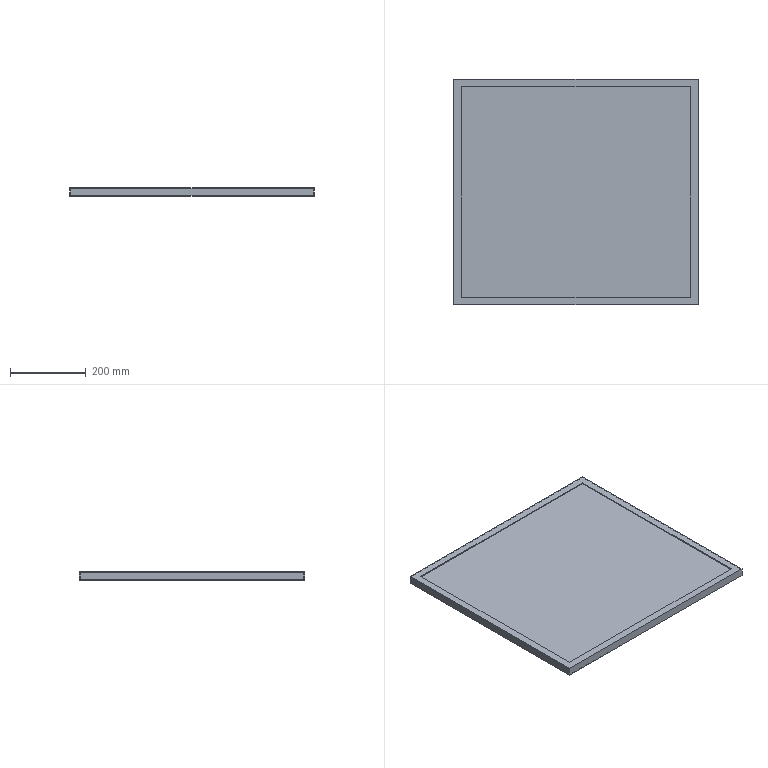Part | SolidWorks | features Extrusion 1, ICE 1, Shell 1 | 1 solid | 16 faces | box 645 x 596 x 22 mm | volume 953984 mm3 | plane 16
STEP:
#1=CARTESIAN_POINT('',(0.,596.,22.));
#2=VERTEX_POINT('',#1);
#3=CARTESIAN_POINT('',(0.,0.,22.));
#4=VERTEX_POINT('',#3);
#5=CARTESIAN_POINT('',(0.,0.,22.));
#6=DIRECTION('',(0.,-1.,0.));
#7=VECTOR('',#6,1000.);
#8=LINE('',#5,#7);
#9=EDGE_CURVE('',#2,#4,#8,.T.);
#10=ORIENTED_EDGE('',*,*,#9,.T.);
#11=CARTESIAN_POINT('',(645.,0.,22.));
#12=VERTEX_POINT('',#11);
#13=CARTESIAN_POINT('',(0.,0.,22.));
#14=DIRECTION('',(1.,0.,0.));
#15=VECTOR('',#14,1000.);
#16=LINE('',#13,#15);
#17=EDGE_CURVE('',#4,#12,#16,.T.);
#18=ORIENTED_EDGE('',*,*,#17,.T.);
#19=CARTESIAN_POINT('',(645.,596.,22.));
#20=VERTEX_POINT('',#19);
#21=CARTESIAN_POINT('',(645.,0.,22.));
#22=DIRECTION('',(0.,1.,0.));
#23=VECTOR('',#22,1000.);
#24=LINE('',#21,#23);
#25=EDGE_CURVE('',#12,#20,#24,.T.);
#26=ORIENTED_EDGE('',*,*,#25,.T.);
#27=CARTESIAN_POINT('',(0.,596.,22.));
#28=DIRECTION('',(-1.,0.,0.));
#29=VECTOR('',#28,1000.);
#30=LINE('',#27,#29);
#31=EDGE_CURVE('',#20,#2,#30,.T.);
#32=ORIENTED_EDGE('',*,*,#31,.T.);
#33=EDGE_LOOP('',(#10,#18,#26,#32));
#34=FACE_OUTER_BOUND('',#33,.T.);
#35=CARTESIAN_POINT('',(625.,576.,22.));
#36=VERTEX_POINT('',#35);
#37=CARTESIAN_POINT('',(20.,576.,22.));
#38=VERTEX_POINT('',#37);
#39=CARTESIAN_POINT('',(625.,576.,22.));
#40=DIRECTION('',(-1.,0.,0.));
#41=VECTOR('',#40,1000.);
#42=LINE('',#39,#41);
#43=EDGE_CURVE('',#36,#38,#42,.T.);
#44=ORIENTED_EDGE('',*,*,#43,.F.);
#45=CARTESIAN_POINT('',(625.,20.,22.));
#46=VERTEX_POINT('',#45);
#47=CARTESIAN_POINT('',(625.,20.,22.));
#48=DIRECTION('',(0.,1.,0.));
#49=VECTOR('',#48,1000.);
#50=LINE('',#47,#49);
#51=EDGE_CURVE('',#46,#36,#50,.T.);
#52=ORIENTED_EDGE('',*,*,#51,.F.);
#53=CARTESIAN_POINT('',(20.,20.,22.));
#54=VERTEX_POINT('',#53);
#55=CARTESIAN_POINT('',(20.,20.,22.));
#56=DIRECTION('',(1.,0.,0.));
#57=VECTOR('',#56,1000.);
#58=LINE('',#55,#57);
#59=EDGE_CURVE('',#54,#46,#58,.T.);
#60=ORIENTED_EDGE('',*,*,#59,.F.);
#61=CARTESIAN_POINT('',(20.,576.,22.));
#62=DIRECTION('',(0.,-1.,0.));
#63=VECTOR('',#62,1000.);
#64=LINE('',#61,#63);
#65=EDGE_CURVE('',#38,#54,#64,.T.);
#66=ORIENTED_EDGE('',*,*,#65,.F.);
#67=EDGE_LOOP('',(#44,#52,#60,#66));
#68=FACE_BOUND('',#67,.T.);
#69=CARTESIAN_POINT('',(0.,596.,22.));
#70=DIRECTION('',(0.,0.,-1.));
#71=DIRECTION('',(-1.,0.,0.));
#72=AXIS2_PLACEMENT_3D('',#69,#70,#71);
#73=PLANE('',#72);
#74=ADVANCED_FACE('',(#34,#68),#73,.F.);
#75=CARTESIAN_POINT('',(0.,596.,0.));
#76=VERTEX_POINT('',#75);
#77=CARTESIAN_POINT('',(0.,596.,22.));
#78=DIRECTION('',(0.,0.,-1.));
#79=VECTOR('',#78,1000.);
#80=LINE('',#77,#79);
#81=EDGE_CURVE('',#2,#76,#80,.T.);
#82=ORIENTED_EDGE('',*,*,#81,.T.);
#83=CARTESIAN_POINT('',(0.,0.,0.));
#84=VERTEX_POINT('',#83);
#85=CARTESIAN_POINT('',(0.,0.,0.));
#86=DIRECTION('',(0.,-1.,0.));
#87=VECTOR('',#86,1000.);
#88=LINE('',#85,#87);
#89=EDGE_CURVE('',#76,#84,#88,.T.);
#90=ORIENTED_EDGE('',*,*,#89,.T.);
#91=CARTESIAN_POINT('',(0.,0.,22.));
#92=DIRECTION('',(0.,0.,-1.));
#93=VECTOR('',#92,1000.);
#94=LINE('',#91,#93);
#95=EDGE_CURVE('',#4,#84,#94,.T.);
#96=ORIENTED_EDGE('',*,*,#95,.F.);
#97=ORIENTED_EDGE('',*,*,#9,.F.);
#98=EDGE_LOOP('',(#82,#90,#96,#97));
#99=FACE_OUTER_BOUND('',#98,.T.);
#100=CARTESIAN_POINT('',(0.,0.,22.));
#101=DIRECTION('',(1.,0.,0.));
#102=DIRECTION('',(0.,0.,-1.));
#103=AXIS2_PLACEMENT_3D('',#100,#101,#102);
#104=PLANE('',#103);
#105=ADVANCED_FACE('',(#99),#104,.F.);
#106=ORIENTED_EDGE('',*,*,#95,.T.);
#107=CARTESIAN_POINT('',(645.,0.,0.));
#108=VERTEX_POINT('',#107);
#109=CARTESIAN_POINT('',(0.,0.,0.));
#110=DIRECTION('',(1.,0.,0.));
#111=VECTOR('',#110,1000.);
#112=LINE('',#109,#111);
#113=EDGE_CURVE('',#84,#108,#112,.T.);
#114=ORIENTED_EDGE('',*,*,#113,.T.);
#115=CARTESIAN_POINT('',(645.,0.,22.));
#116=DIRECTION('',(0.,0.,-1.));
#117=VECTOR('',#116,1000.);
#118=LINE('',#115,#117);
#119=EDGE_CURVE('',#12,#108,#118,.T.);
#120=ORIENTED_EDGE('',*,*,#119,.F.);
#121=ORIENTED_EDGE('',*,*,#17,.F.);
#122=EDGE_LOOP('',(#106,#114,#120,#121));
#123=FACE_OUTER_BOUND('',#122,.T.);
#124=CARTESIAN_POINT('',(0.,0.,22.));
#125=DIRECTION('',(0.,1.,0.));
#126=DIRECTION('',(0.,0.,1.));
#127=AXIS2_PLACEMENT_3D('',#124,#125,#126);
#128=PLANE('',#127);
#129=ADVANCED_FACE('',(#123),#128,.F.);
#130=ORIENTED_EDGE('',*,*,#119,.T.);
#131=CARTESIAN_POINT('',(645.,596.,0.));
#132=VERTEX_POINT('',#131);
#133=CARTESIAN_POINT('',(645.,0.,0.));
#134=DIRECTION('',(0.,1.,0.));
#135=VECTOR('',#134,1000.);
#136=LINE('',#133,#135);
#137=EDGE_CURVE('',#108,#132,#136,.T.);
#138=ORIENTED_EDGE('',*,*,#137,.T.);
#139=CARTESIAN_POINT('',(645.,596.,22.));
#140=DIRECTION('',(0.,0.,-1.));
#141=VECTOR('',#140,1000.);
#142=LINE('',#139,#141);
#143=EDGE_CURVE('',#20,#132,#142,.T.);
#144=ORIENTED_EDGE('',*,*,#143,.F.);
#145=ORIENTED_EDGE('',*,*,#25,.F.);
#146=EDGE_LOOP('',(#130,#138,#144,#145));
#147=FACE_OUTER_BOUND('',#146,.T.);
#148=CARTESIAN_POINT('',(645.,0.,22.));
#149=DIRECTION('',(-1.,0.,0.));
#150=DIRECTION('',(0.,0.,1.));
#151=AXIS2_PLACEMENT_3D('',#148,#149,#150);
#152=PLANE('',#151);
#153=ADVANCED_FACE('',(#147),#152,.F.);
#154=ORIENTED_EDGE('',*,*,#143,.T.);
#155=CARTESIAN_POINT('',(0.,596.,0.));
#156=DIRECTION('',(-1.,0.,0.));
#157=VECTOR('',#156,1000.);
#158=LINE('',#155,#157);
#159=EDGE_CURVE('',#132,#76,#158,.T.);
#160=ORIENTED_EDGE('',*,*,#159,.T.);
#161=ORIENTED_EDGE('',*,*,#81,.F.);
#162=ORIENTED_EDGE('',*,*,#31,.F.);
#163=EDGE_LOOP('',(#154,#160,#161,#162));
#164=FACE_OUTER_BOUND('',#163,.T.);
#165=CARTESIAN_POINT('',(0.,596.,22.));
#166=DIRECTION('',(0.,-1.,0.));
#167=DIRECTION('',(0.,0.,-1.));
#168=AXIS2_PLACEMENT_3D('',#165,#166,#167);
#169=PLANE('',#168);
#170=ADVANCED_FACE('',(#164),#169,.F.);
#171=ORIENTED_EDGE('',*,*,#89,.F.);
#172=ORIENTED_EDGE('',*,*,#159,.F.);
#173=ORIENTED_EDGE('',*,*,#137,.F.);
#174=ORIENTED_EDGE('',*,*,#113,.F.);
#175=EDGE_LOOP('',(#171,#172,#173,#174));
#176=FACE_OUTER_BOUND('',#175,.T.);
#177=CARTESIAN_POINT('',(0.,596.,0.));
#178=DIRECTION('',(0.,0.,-1.));
#179=DIRECTION('',(-1.,0.,0.));
#180=AXIS2_PLACEMENT_3D('',#177,#178,#179);
#181=PLANE('',#180);
#182=ADVANCED_FACE('',(#176),#181,.T.);
#183=CARTESIAN_POINT('',(2.,594.,20.));
#184=VERTEX_POINT('',#183);
#185=CARTESIAN_POINT('',(2.,2.,20.));
#186=VERTEX_POINT('',#185);
#187=CARTESIAN_POINT('',(2.,0.,20.));
#188=DIRECTION('',(0.,-1.,0.));
#189=VECTOR('',#188,1000.);
#190=LINE('',#187,#189);
#191=EDGE_CURVE('',#184,#186,#190,.T.);
#192=ORIENTED_EDGE('',*,*,#191,.F.);
#193=CARTESIAN_POINT('',(643.,594.,20.));
#194=VERTEX_POINT('',#193);
#195=CARTESIAN_POINT('',(0.,594.,20.));
#196=DIRECTION('',(-1.,0.,0.));
#197=VECTOR('',#196,1000.);
#198=LINE('',#195,#197);
#199=EDGE_CURVE('',#194,#184,#198,.T.);
#200=ORIENTED_EDGE('',*,*,#199,.F.);
#201=CARTESIAN_POINT('',(643.,2.,20.));
#202=VERTEX_POINT('',#201);
#203=CARTESIAN_POINT('',(643.,0.,20.));
#204=DIRECTION('',(0.,1.,0.));
#205=VECTOR('',#204,1000.);
#206=LINE('',#203,#205);
#207=EDGE_CURVE('',#202,#194,#206,.T.);
#208=ORIENTED_EDGE('',*,*,#207,.F.);
#209=CARTESIAN_POINT('',(0.,2.,20.));
#210=DIRECTION('',(1.,0.,0.));
#211=VECTOR('',#210,1000.);
#212=LINE('',#209,#211);
#213=EDGE_CURVE('',#186,#202,#212,.T.);
#214=ORIENTED_EDGE('',*,*,#213,.F.);
#215=EDGE_LOOP('',(#192,#200,#208,#214));
#216=FACE_OUTER_BOUND('',#215,.T.);
#217=CARTESIAN_POINT('',(625.,20.,20.));
#218=VERTEX_POINT('',#217);
#219=CARTESIAN_POINT('',(625.,576.,20.));
#220=VERTEX_POINT('',#219);
#221=CARTESIAN_POINT('',(625.,20.,20.));
#222=DIRECTION('',(0.,1.,0.));
#223=VECTOR('',#222,1000.);
#224=LINE('',#221,#223);
#225=EDGE_CURVE('',#218,#220,#224,.T.);
#226=ORIENTED_EDGE('',*,*,#225,.T.);
#227=CARTESIAN_POINT('',(20.,576.,20.));
#228=VERTEX_POINT('',#227);
#229=CARTESIAN_POINT('',(625.,576.,20.));
#230=DIRECTION('',(-1.,0.,0.));
#231=VECTOR('',#230,1000.);
#232=LINE('',#229,#231);
#233=EDGE_CURVE('',#220,#228,#232,.T.);
#234=ORIENTED_EDGE('',*,*,#233,.T.);
#235=CARTESIAN_POINT('',(20.,20.,20.));
#236=VERTEX_POINT('',#235);
#237=CARTESIAN_POINT('',(20.,576.,20.));
#238=DIRECTION('',(0.,-1.,0.));
#239=VECTOR('',#238,1000.);
#240=LINE('',#237,#239);
#241=EDGE_CURVE('',#228,#236,#240,.T.);
#242=ORIENTED_EDGE('',*,*,#241,.T.);
#243=CARTESIAN_POINT('',(20.,20.,20.));
#244=DIRECTION('',(1.,0.,0.));
#245=VECTOR('',#244,1000.);
#246=LINE('',#243,#245);
#247=EDGE_CURVE('',#236,#218,#246,.T.);
#248=ORIENTED_EDGE('',*,*,#247,.T.);
#249=EDGE_LOOP('',(#226,#234,#242,#248));
#250=FACE_BOUND('',#249,.T.);
#251=CARTESIAN_POINT('',(0.,596.,20.));
#252=DIRECTION('',(0.,0.,1.));
#253=DIRECTION('',(1.,0.,0.));
#254=AXIS2_PLACEMENT_3D('',#251,#252,#253);
#255=PLANE('',#254);
#256=ADVANCED_FACE('',(#216,#250),#255,.F.);
#257=ORIENTED_EDGE('',*,*,#43,.T.);
#258=CARTESIAN_POINT('',(20.,576.,20.));
#259=DIRECTION('',(0.,0.,1.));
#260=VECTOR('',#259,1000.);
#261=LINE('',#258,#260);
#262=EDGE_CURVE('',#228,#38,#261,.T.);
#263=ORIENTED_EDGE('',*,*,#262,.F.);
#264=ORIENTED_EDGE('',*,*,#233,.F.);
#265=CARTESIAN_POINT('',(625.,576.,20.));
#266=DIRECTION('',(0.,0.,1.));
#267=VECTOR('',#266,1000.);
#268=LINE('',#265,#267);
#269=EDGE_CURVE('',#220,#36,#268,.T.);
#270=ORIENTED_EDGE('',*,*,#269,.T.);
#271=EDGE_LOOP('',(#257,#263,#264,#270));
#272=FACE_OUTER_BOUND('',#271,.T.);
#273=CARTESIAN_POINT('',(625.,576.,20.));
#274=DIRECTION('',(0.,1.,0.));
#275=DIRECTION('',(0.,0.,1.));
#276=AXIS2_PLACEMENT_3D('',#273,#274,#275);
#277=PLANE('',#276);
#278=ADVANCED_FACE('',(#272),#277,.F.);
#279=ORIENTED_EDGE('',*,*,#51,.T.);
#280=ORIENTED_EDGE('',*,*,#269,.F.);
#281=ORIENTED_EDGE('',*,*,#225,.F.);
#282=CARTESIAN_POINT('',(625.,20.,20.));
#283=DIRECTION('',(0.,0.,1.));
#284=VECTOR('',#283,1000.);
#285=LINE('',#282,#284);
#286=EDGE_CURVE('',#218,#46,#285,.T.);
#287=ORIENTED_EDGE('',*,*,#286,.T.);
#288=EDGE_LOOP('',(#279,#280,#281,#287));
#289=FACE_OUTER_BOUND('',#288,.T.);
#290=CARTESIAN_POINT('',(625.,20.,20.));
#291=DIRECTION('',(1.,0.,0.));
#292=DIRECTION('',(0.,0.,-1.));
#293=AXIS2_PLACEMENT_3D('',#290,#291,#292);
#294=PLANE('',#293);
#295=ADVANCED_FACE('',(#289),#294,.F.);
#296=ORIENTED_EDGE('',*,*,#59,.T.);
#297=ORIENTED_EDGE('',*,*,#286,.F.);
#298=ORIENTED_EDGE('',*,*,#247,.F.);
#299=CARTESIAN_POINT('',(20.,20.,20.));
#300=DIRECTION('',(0.,0.,1.));
#301=VECTOR('',#300,1000.);
#302=LINE('',#299,#301);
#303=EDGE_CURVE('',#236,#54,#302,.T.);
#304=ORIENTED_EDGE('',*,*,#303,.T.);
#305=EDGE_LOOP('',(#296,#297,#298,#304));
#306=FACE_OUTER_BOUND('',#305,.T.);
#307=CARTESIAN_POINT('',(20.,20.,20.));
#308=DIRECTION('',(0.,-1.,0.));
#309=DIRECTION('',(0.,0.,-1.));
#310=AXIS2_PLACEMENT_3D('',#307,#308,#309);
#311=PLANE('',#310);
#312=ADVANCED_FACE('',(#306),#311,.F.);
#313=ORIENTED_EDGE('',*,*,#65,.T.);
#314=ORIENTED_EDGE('',*,*,#303,.F.);
#315=ORIENTED_EDGE('',*,*,#241,.F.);
#316=ORIENTED_EDGE('',*,*,#262,.T.);
#317=EDGE_LOOP('',(#313,#314,#315,#316));
#318=FACE_OUTER_BOUND('',#317,.T.);
#319=CARTESIAN_POINT('',(20.,576.,20.));
#320=DIRECTION('',(-1.,0.,0.));
#321=DIRECTION('',(0.,0.,1.));
#322=AXIS2_PLACEMENT_3D('',#319,#320,#321);
#323=PLANE('',#322);
#324=ADVANCED_FACE('',(#318),#323,.F.);
#325=CARTESIAN_POINT('',(2.,594.,2.));
#326=VERTEX_POINT('',#325);
#327=CARTESIAN_POINT('',(2.,2.,2.));
#328=VERTEX_POINT('',#327);
#329=CARTESIAN_POINT('',(2.,596.,2.));
#330=DIRECTION('',(0.,-1.,0.));
#331=VECTOR('',#330,1000.);
#332=LINE('',#329,#331);
#333=EDGE_CURVE('',#326,#328,#332,.T.);
#334=ORIENTED_EDGE('',*,*,#333,.T.);
#335=CARTESIAN_POINT('',(643.,2.,2.));
#336=VERTEX_POINT('',#335);
#337=CARTESIAN_POINT('',(0.,2.,2.));
#338=DIRECTION('',(1.,0.,0.));
#339=VECTOR('',#338,1000.);
#340=LINE('',#337,#339);
#341=EDGE_CURVE('',#328,#336,#340,.T.);
#342=ORIENTED_EDGE('',*,*,#341,.T.);
#343=CARTESIAN_POINT('',(643.,594.,2.));
#344=VERTEX_POINT('',#343);
#345=CARTESIAN_POINT('',(643.,596.,2.));
#346=DIRECTION('',(0.,1.,0.));
#347=VECTOR('',#346,1000.);
#348=LINE('',#345,#347);
#349=EDGE_CURVE('',#336,#344,#348,.T.);
#350=ORIENTED_EDGE('',*,*,#349,.T.);
#351=CARTESIAN_POINT('',(0.,594.,2.));
#352=DIRECTION('',(-1.,0.,0.));
#353=VECTOR('',#352,1000.);
#354=LINE('',#351,#353);
#355=EDGE_CURVE('',#344,#326,#354,.T.);
#356=ORIENTED_EDGE('',*,*,#355,.T.);
#357=EDGE_LOOP('',(#334,#342,#350,#356));
#358=FACE_OUTER_BOUND('',#357,.T.);
#359=CARTESIAN_POINT('',(0.,596.,2.));
#360=DIRECTION('',(0.,0.,-1.));
#361=DIRECTION('',(-1.,0.,0.));
#362=AXIS2_PLACEMENT_3D('',#359,#360,#361);
#363=PLANE('',#362);
#364=ADVANCED_FACE('',(#358),#363,.F.);
#365=CARTESIAN_POINT('',(643.,594.,22.));
#366=DIRECTION('',(0.,0.,-1.));
#367=VECTOR('',#366,1000.);
#368=LINE('',#365,#367);
#369=EDGE_CURVE('',#194,#344,#368,.T.);
#370=ORIENTED_EDGE('',*,*,#369,.F.);
#371=ORIENTED_EDGE('',*,*,#199,.T.);
#372=CARTESIAN_POINT('',(2.,594.,22.));
#373=DIRECTION('',(0.,0.,-1.));
#374=VECTOR('',#373,1000.);
#375=LINE('',#372,#374);
#376=EDGE_CURVE('',#184,#326,#375,.T.);
#377=ORIENTED_EDGE('',*,*,#376,.T.);
#378=ORIENTED_EDGE('',*,*,#355,.F.);
#379=EDGE_LOOP('',(#370,#371,#377,#378));
#380=FACE_OUTER_BOUND('',#379,.T.);
#381=CARTESIAN_POINT('',(0.,594.,22.));
#382=DIRECTION('',(0.,-1.,0.));
#383=DIRECTION('',(0.,0.,-1.));
#384=AXIS2_PLACEMENT_3D('',#381,#382,#383);
#385=PLANE('',#384);
#386=ADVANCED_FACE('',(#380),#385,.T.);
#387=CARTESIAN_POINT('',(643.,2.,22.));
#388=DIRECTION('',(0.,0.,-1.));
#389=VECTOR('',#388,1000.);
#390=LINE('',#387,#389);
#391=EDGE_CURVE('',#202,#336,#390,.T.);
#392=ORIENTED_EDGE('',*,*,#391,.F.);
#393=ORIENTED_EDGE('',*,*,#207,.T.);
#394=ORIENTED_EDGE('',*,*,#369,.T.);
#395=ORIENTED_EDGE('',*,*,#349,.F.);
#396=EDGE_LOOP('',(#392,#393,#394,#395));
#397=FACE_OUTER_BOUND('',#396,.T.);
#398=CARTESIAN_POINT('',(643.,0.,22.));
#399=DIRECTION('',(-1.,0.,0.));
#400=DIRECTION('',(0.,0.,1.));
#401=AXIS2_PLACEMENT_3D('',#398,#399,#400);
#402=PLANE('',#401);
#403=ADVANCED_FACE('',(#397),#402,.T.);
#404=CARTESIAN_POINT('',(2.,2.,22.));
#405=DIRECTION('',(0.,0.,-1.));
#406=VECTOR('',#405,1000.);
#407=LINE('',#404,#406);
#408=EDGE_CURVE('',#186,#328,#407,.T.);
#409=ORIENTED_EDGE('',*,*,#408,.F.);
#410=ORIENTED_EDGE('',*,*,#213,.T.);
#411=ORIENTED_EDGE('',*,*,#391,.T.);
#412=ORIENTED_EDGE('',*,*,#341,.F.);
#413=EDGE_LOOP('',(#409,#410,#411,#412));
#414=FACE_OUTER_BOUND('',#413,.T.);
#415=CARTESIAN_POINT('',(0.,2.,22.));
#416=DIRECTION('',(0.,1.,0.));
#417=DIRECTION('',(0.,0.,1.));
#418=AXIS2_PLACEMENT_3D('',#415,#416,#417);
#419=PLANE('',#418);
#420=ADVANCED_FACE('',(#414),#419,.T.);
#421=ORIENTED_EDGE('',*,*,#376,.F.);
#422=ORIENTED_EDGE('',*,*,#191,.T.);
#423=ORIENTED_EDGE('',*,*,#408,.T.);
#424=ORIENTED_EDGE('',*,*,#333,.F.);
#425=EDGE_LOOP('',(#421,#422,#423,#424));
#426=FACE_OUTER_BOUND('',#425,.T.);
#427=CARTESIAN_POINT('',(2.,0.,22.));
#428=DIRECTION('',(1.,0.,0.));
#429=DIRECTION('',(0.,0.,-1.));
#430=AXIS2_PLACEMENT_3D('',#427,#428,#429);
#431=PLANE('',#430);
#432=ADVANCED_FACE('',(#426),#431,.T.);
#433=CLOSED_SHELL('',(#74,#105,#129,#153,#170,#182,#256,#278,#295,#312,#324,#364,#386,#403,#420,#432));
#434=MANIFOLD_SOLID_BREP('',#433);
#435=CARTESIAN_POINT('',(0.,0.,0.));
#436=DIRECTION('',(0.,0.,1.));
#437=DIRECTION('',(1.,0.,0.));
#438=AXIS2_PLACEMENT_3D('',#435,#436,#437);
#439=(LENGTH_UNIT()NAMED_UNIT(*)SI_UNIT(.MILLI.,.METRE.));
#440=UNCERTAINTY_MEASURE_WITH_UNIT(LENGTH_MEASURE(0.00001),#439,'','');
#441=(NAMED_UNIT(*)PLANE_ANGLE_UNIT()SI_UNIT($,.RADIAN.));
#442=(NAMED_UNIT(*)SI_UNIT($,.STERADIAN.)SOLID_ANGLE_UNIT());
#443=(GEOMETRIC_REPRESENTATION_CONTEXT(3)GLOBAL_UNCERTAINTY_ASSIGNED_CONTEXT((#440))GLOBAL_UNIT_ASSIGNED_CONTEXT((#439,#441,#442))REPRESENTATION_CONTEXT('',''));
#444=ADVANCED_BREP_SHAPE_REPRESENTATION('',(#434,#438),#443);